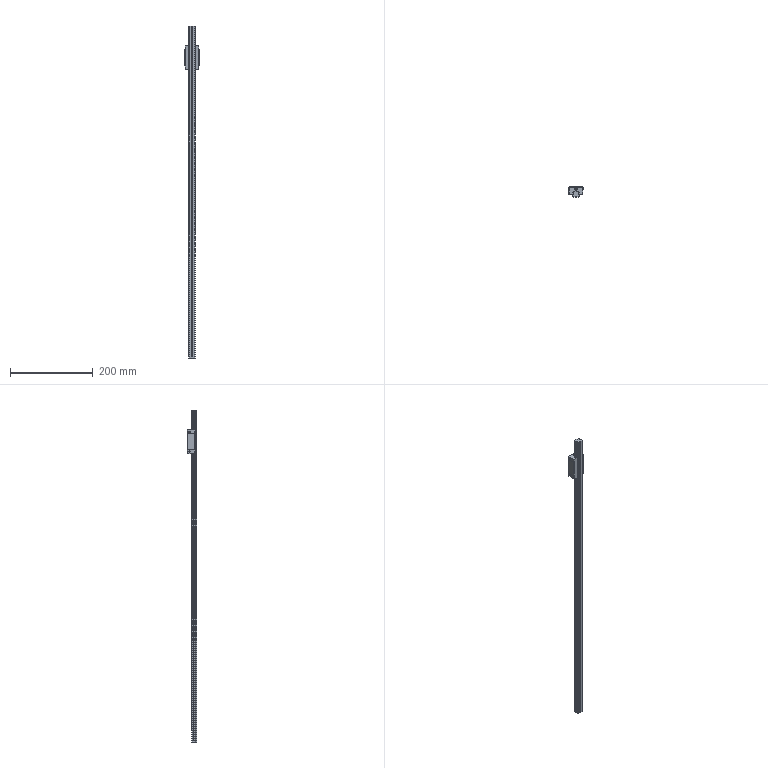Part | SolidWorks | 2 solids | 232 faces | box 34 x 24 x 801 mm | volume 156547 mm3 | cylinder 120 | plane 112 | commonest cylinder face diameters 4.5 x26 8 x26 0.6 x12 4 x12 3 x10 0.46 x8